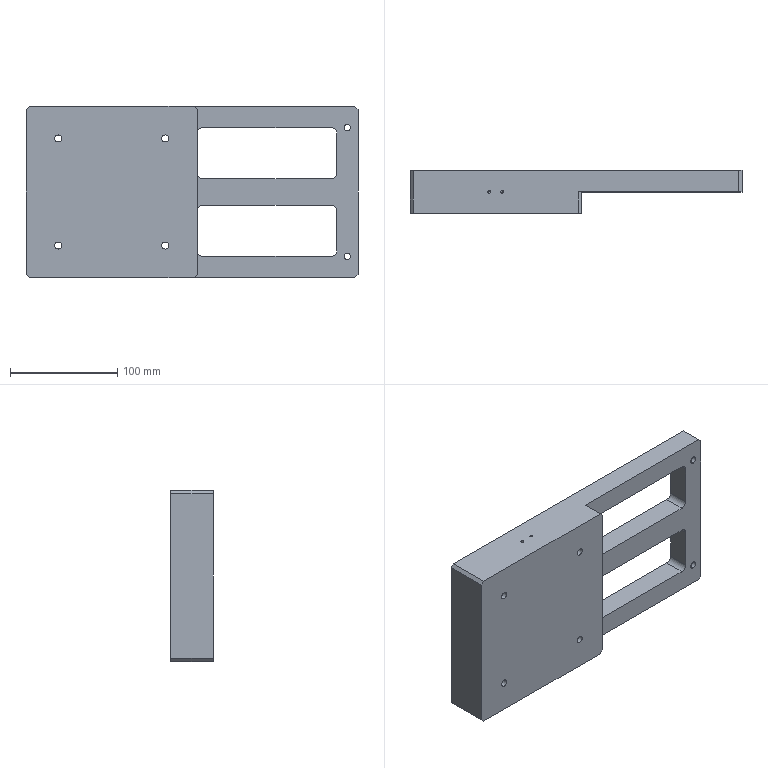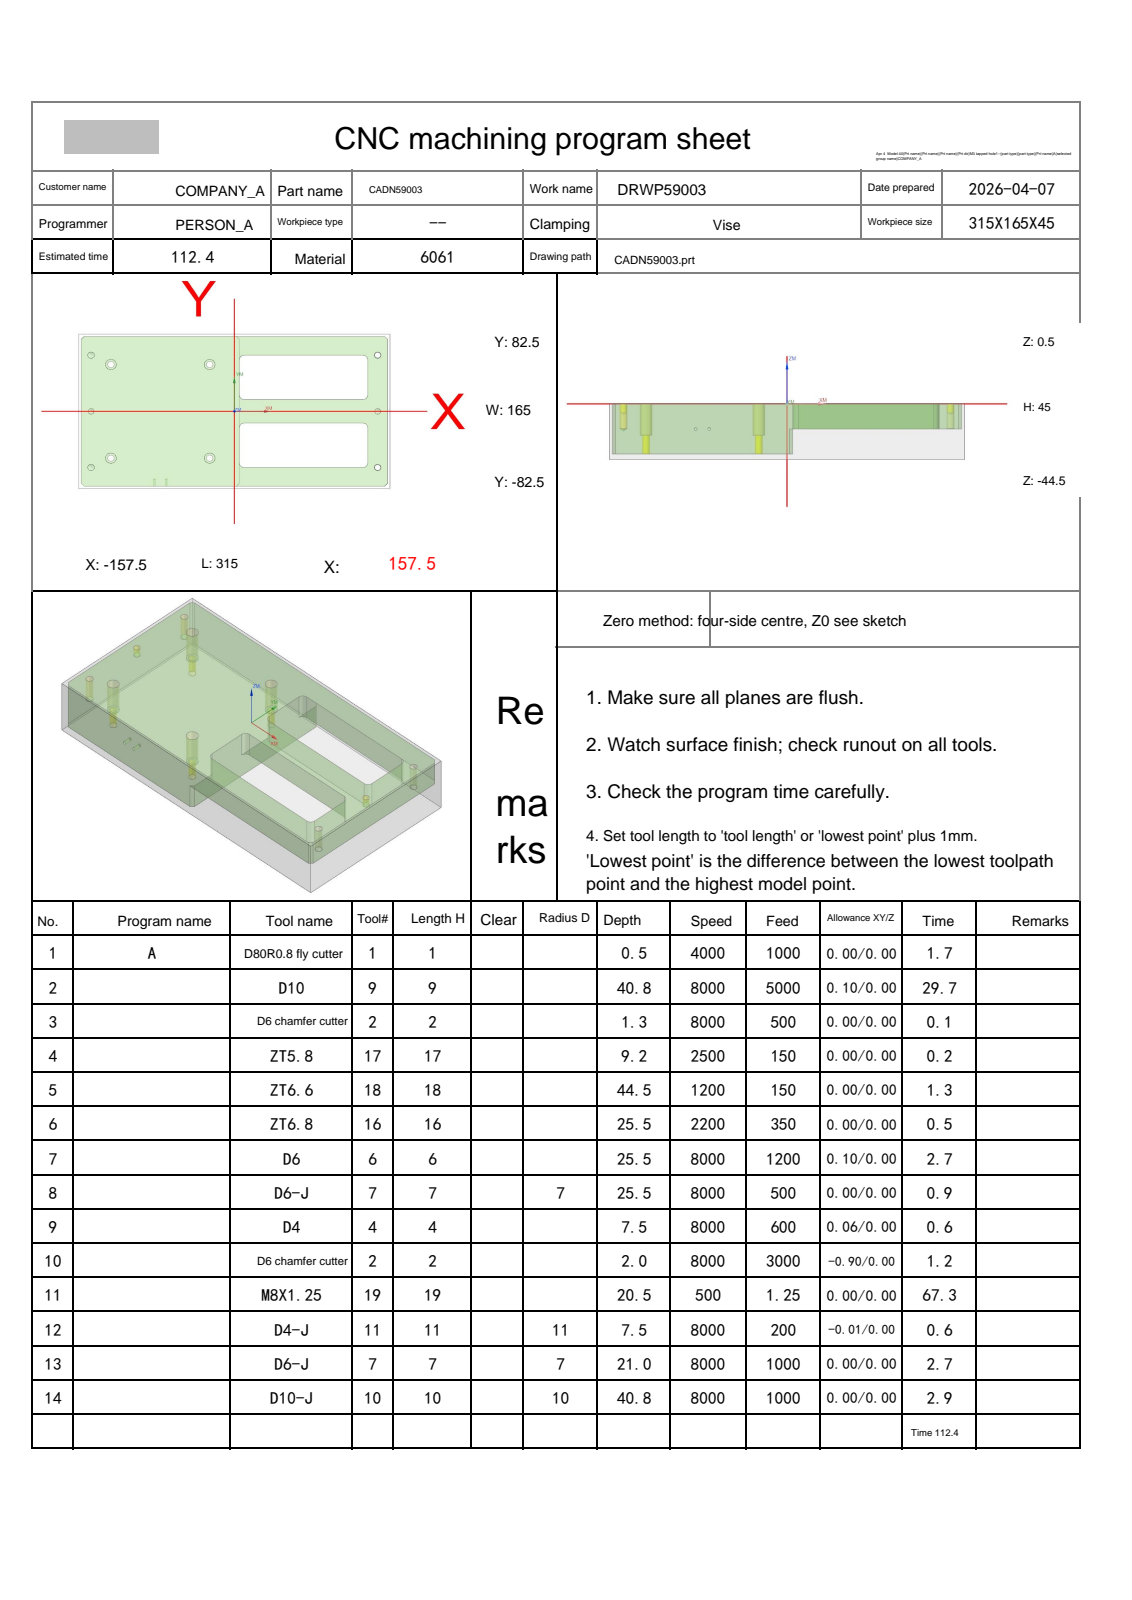NC program | NX | posted by the shop | part box 310 x 40 x 160 mm
Lines 1 to 44 of 5464:
%
O0001
(Machine time: 179.09 MIN)
(===Total Tool:12===)
(T1=D80R0.8 fly cutter D=80.  R=0.8  D-  H01 Z=-0.   )
(T9=D10     D=10.  R=0.   D-  H09 Z=-40.3 )
(T2=D6 chamfer cutter   D=6.   R=0.   D-  H02 Z=-1.5  )
(T17=ZT5.8  D=5.8  DR_a=118 D-  H17 Z=-8.7  )
(T18=ZT6.6  D=6.6  DR_a=118 D-  H18 Z=-43.98)
(T16=ZT6.8  D=6.8  DR_a=118 D-  H16 Z=-25.  )
(T6=D6      D=6.   R=0.   D-  H06 Z=-25.  )
(T7=D6-J    D=6.   R=0.   D7  H07 Z=-25.  )
(T4=D4      D=4.   R=0.   D-  H04 Z=-7.   )
(T19=M8X1.25 D=6.8  DR_a=180 D-  H19 Z=-20.  )
(T11=D4-J   D=4.   R=0.   D11 H11 Z=-7.   )
(T10=D10-J  D=10.  R=0.   D10 H10 Z=-40.3 )
G80 G90 G17 G49 G40
G91 G28 Z0
M01
N1 T01 M06
(D80R0.8 fly cutter  D=80. R=0.8 H=01 ce=0.00 di=0.00)
G00 G90 G54 X200. Y-72. M03 S4000
G43 H01 Z20.
M08
Z2.
G01 Z0.0 F1000.
X195.
X-195.
Y-24.
X195.
Y24.
X-195.
Y72.
X195.
X200.
Z2.
G00 Z20.
G91 G28 Z0.0
M05
M09
G91 G28 Z0.0
M01